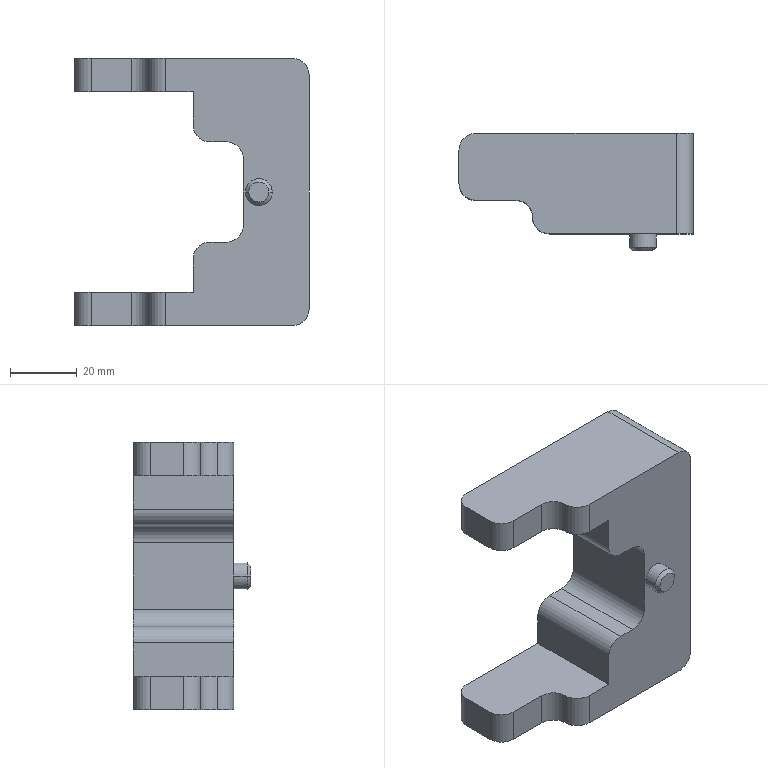Part | NX | features BREP 1 | 1 solid | 36 faces | box 70 x 35 x 80 mm | volume 86102 mm3 | plane 17 | cylinder 16 | cone 3 | commonest cylinder face diameters 10 x14 8 x2
STEP:
#1=CARTESIAN_POINT('',(-8.,0.,30.05));
#2=VERTEX_POINT('',#1);
#3=CARTESIAN_POINT('',(0.3433,0.,30.05));
#4=VERTEX_POINT('',#3);
#5=CARTESIAN_POINT('',(-8.,0.,30.05));
#6=DIRECTION('',(1.,0.,0.));
#7=VECTOR('',#6,1000.);
#8=LINE('',#5,#7);
#9=EDGE_CURVE('',#2,#4,#8,.T.);
#10=ORIENTED_EDGE('',*,*,#9,.T.);
#11=CARTESIAN_POINT('',(0.3433,0.,20.));
#12=VERTEX_POINT('',#11);
#13=CARTESIAN_POINT('',(0.3433,0.,30.05));
#14=DIRECTION('',(0.,0.,-1.));
#15=VECTOR('',#14,1000.);
#16=LINE('',#13,#15);
#17=EDGE_CURVE('',#4,#12,#16,.T.);
#18=ORIENTED_EDGE('',*,*,#17,.T.);
#19=CARTESIAN_POINT('',(5.343,0.,15.));
#20=VERTEX_POINT('',#19);
#21=CARTESIAN_POINT('',(5.343,0.,20.));
#22=DIRECTION('',(0.,-1.,0.));
#23=DIRECTION('',(-1.,0.,0.));
#24=AXIS2_PLACEMENT_3D('',#21,#22,#23);
#25=CIRCLE('',#24,5.);
#26=EDGE_CURVE('',#12,#20,#25,.T.);
#27=ORIENTED_EDGE('',*,*,#26,.T.);
#28=CARTESIAN_POINT('',(10.343,0.,15.));
#29=VERTEX_POINT('',#28);
#30=CARTESIAN_POINT('',(5.343,0.,15.));
#31=DIRECTION('',(1.,0.,0.));
#32=VECTOR('',#31,1000.);
#33=LINE('',#30,#32);
#34=EDGE_CURVE('',#20,#29,#33,.T.);
#35=ORIENTED_EDGE('',*,*,#34,.T.);
#36=CARTESIAN_POINT('',(15.343,0.,10.));
#37=VERTEX_POINT('',#36);
#38=CARTESIAN_POINT('',(10.343,0.,10.));
#39=DIRECTION('',(0.,1.,0.));
#40=DIRECTION('',(0.,0.,1.));
#41=AXIS2_PLACEMENT_3D('',#38,#39,#40);
#42=CIRCLE('',#41,5.);
#43=EDGE_CURVE('',#29,#37,#42,.T.);
#44=ORIENTED_EDGE('',*,*,#43,.T.);
#45=CARTESIAN_POINT('',(15.343,0.,-10.));
#46=VERTEX_POINT('',#45);
#47=CARTESIAN_POINT('',(15.343,0.,10.));
#48=DIRECTION('',(0.,0.,-1.));
#49=VECTOR('',#48,1000.);
#50=LINE('',#47,#49);
#51=EDGE_CURVE('',#37,#46,#50,.T.);
#52=ORIENTED_EDGE('',*,*,#51,.T.);
#53=CARTESIAN_POINT('',(10.343,0.,-15.));
#54=VERTEX_POINT('',#53);
#55=CARTESIAN_POINT('',(10.343,0.,-10.));
#56=DIRECTION('',(0.,1.,0.));
#57=DIRECTION('',(1.,0.,0.));
#58=AXIS2_PLACEMENT_3D('',#55,#56,#57);
#59=CIRCLE('',#58,5.);
#60=EDGE_CURVE('',#46,#54,#59,.T.);
#61=ORIENTED_EDGE('',*,*,#60,.T.);
#62=CARTESIAN_POINT('',(5.343,0.,-15.));
#63=VERTEX_POINT('',#62);
#64=CARTESIAN_POINT('',(10.343,0.,-15.));
#65=DIRECTION('',(-1.,0.,0.));
#66=VECTOR('',#65,1000.);
#67=LINE('',#64,#66);
#68=EDGE_CURVE('',#54,#63,#67,.T.);
#69=ORIENTED_EDGE('',*,*,#68,.T.);
#70=CARTESIAN_POINT('',(0.3433,0.,-20.));
#71=VERTEX_POINT('',#70);
#72=CARTESIAN_POINT('',(5.343,0.,-20.));
#73=DIRECTION('',(0.,-1.,0.));
#74=DIRECTION('',(0.,0.,1.));
#75=AXIS2_PLACEMENT_3D('',#72,#73,#74);
#76=CIRCLE('',#75,5.);
#77=EDGE_CURVE('',#63,#71,#76,.T.);
#78=ORIENTED_EDGE('',*,*,#77,.T.);
#79=CARTESIAN_POINT('',(0.3433,0.,-30.05));
#80=VERTEX_POINT('',#79);
#81=CARTESIAN_POINT('',(0.3433,0.,-20.));
#82=DIRECTION('',(0.,0.,-1.));
#83=VECTOR('',#82,1000.);
#84=LINE('',#81,#83);
#85=EDGE_CURVE('',#71,#80,#84,.T.);
#86=ORIENTED_EDGE('',*,*,#85,.T.);
#87=CARTESIAN_POINT('',(-8.,0.,-30.05));
#88=VERTEX_POINT('',#87);
#89=CARTESIAN_POINT('',(-8.,0.,-30.05));
#90=DIRECTION('',(1.,0.,0.));
#91=VECTOR('',#90,1000.);
#92=LINE('',#89,#91);
#93=EDGE_CURVE('',#88,#80,#92,.T.);
#94=ORIENTED_EDGE('',*,*,#93,.F.);
#95=CARTESIAN_POINT('',(-8.,0.,-40.));
#96=VERTEX_POINT('',#95);
#97=CARTESIAN_POINT('',(-8.,0.,-30.05));
#98=DIRECTION('',(0.,0.,-1.));
#99=VECTOR('',#98,1000.);
#100=LINE('',#97,#99);
#101=EDGE_CURVE('',#88,#96,#100,.T.);
#102=ORIENTED_EDGE('',*,*,#101,.T.);
#103=CARTESIAN_POINT('',(30.,0.,-40.));
#104=VERTEX_POINT('',#103);
#105=CARTESIAN_POINT('',(30.,0.,-40.));
#106=DIRECTION('',(-1.,0.,0.));
#107=VECTOR('',#106,1000.);
#108=LINE('',#105,#107);
#109=EDGE_CURVE('',#104,#96,#108,.T.);
#110=ORIENTED_EDGE('',*,*,#109,.F.);
#111=CARTESIAN_POINT('',(35.,0.,-35.));
#112=VERTEX_POINT('',#111);
#113=CARTESIAN_POINT('',(30.,0.,-35.));
#114=DIRECTION('',(0.,-1.,0.));
#115=DIRECTION('',(0.,0.,-1.));
#116=AXIS2_PLACEMENT_3D('',#113,#114,#115);
#117=CIRCLE('',#116,5.);
#118=EDGE_CURVE('',#104,#112,#117,.T.);
#119=ORIENTED_EDGE('',*,*,#118,.T.);
#120=CARTESIAN_POINT('',(35.,0.,35.));
#121=VERTEX_POINT('',#120);
#122=CARTESIAN_POINT('',(35.,0.,35.));
#123=DIRECTION('',(0.,0.,-1.));
#124=VECTOR('',#123,1000.);
#125=LINE('',#122,#124);
#126=EDGE_CURVE('',#121,#112,#125,.T.);
#127=ORIENTED_EDGE('',*,*,#126,.F.);
#128=CARTESIAN_POINT('',(30.,0.,40.));
#129=VERTEX_POINT('',#128);
#130=CARTESIAN_POINT('',(30.,0.,35.));
#131=DIRECTION('',(0.,-1.,0.));
#132=DIRECTION('',(1.,0.,0.));
#133=AXIS2_PLACEMENT_3D('',#130,#131,#132);
#134=CIRCLE('',#133,5.);
#135=EDGE_CURVE('',#121,#129,#134,.T.);
#136=ORIENTED_EDGE('',*,*,#135,.T.);
#137=CARTESIAN_POINT('',(-8.,0.,40.));
#138=VERTEX_POINT('',#137);
#139=CARTESIAN_POINT('',(-8.,0.,40.));
#140=DIRECTION('',(1.,0.,0.));
#141=VECTOR('',#140,1000.);
#142=LINE('',#139,#141);
#143=EDGE_CURVE('',#138,#129,#142,.T.);
#144=ORIENTED_EDGE('',*,*,#143,.F.);
#145=CARTESIAN_POINT('',(-8.,0.,40.));
#146=DIRECTION('',(0.,0.,-1.));
#147=VECTOR('',#146,1000.);
#148=LINE('',#145,#147);
#149=EDGE_CURVE('',#138,#2,#148,.T.);
#150=ORIENTED_EDGE('',*,*,#149,.T.);
#151=EDGE_LOOP('',(#10,#18,#27,#35,#44,#52,#61,#69,#78,#86,#94,#102,#110,#119,#127,#136,#144,#150));
#152=FACE_BOUND('',#151,.T.);
#153=CARTESIAN_POINT('',(16.,0.,0.));
#154=VERTEX_POINT('',#153);
#155=CARTESIAN_POINT('',(24.,0.,0.));
#156=VERTEX_POINT('',#155);
#157=CARTESIAN_POINT('',(20.,0.,0.));
#158=DIRECTION('',(0.,1.,0.));
#159=DIRECTION('',(-1.,0.,0.));
#160=AXIS2_PLACEMENT_3D('',#157,#158,#159);
#161=CIRCLE('',#160,4.);
#162=EDGE_CURVE('',#154,#156,#161,.T.);
#163=ORIENTED_EDGE('',*,*,#162,.T.);
#164=CARTESIAN_POINT('',(20.,0.,0.));
#165=DIRECTION('',(0.,1.,0.));
#166=DIRECTION('',(1.,0.,0.));
#167=AXIS2_PLACEMENT_3D('',#164,#165,#166);
#168=CIRCLE('',#167,4.);
#169=EDGE_CURVE('',#156,#154,#168,.T.);
#170=ORIENTED_EDGE('',*,*,#169,.T.);
#171=EDGE_LOOP('',(#163,#170));
#172=FACE_BOUND('',#171,.T.);
#173=CARTESIAN_POINT('',(0.,0.,0.));
#174=DIRECTION('',(0.,1.,0.));
#175=DIRECTION('',(1.,0.,0.));
#176=AXIS2_PLACEMENT_3D('',#173,#174,#175);
#177=PLANE('',#176);
#178=ADVANCED_FACE('',(#152,#172),#177,.F.);
#179=CARTESIAN_POINT('',(16.,-4.,0.));
#180=VERTEX_POINT('',#179);
#181=CARTESIAN_POINT('',(16.,0.,0.));
#182=DIRECTION('',(0.000000001,-1.,-0.000000003));
#183=VECTOR('',#182,1000.);
#184=LINE('',#181,#183);
#185=EDGE_CURVE('',#154,#180,#184,.T.);
#186=ORIENTED_EDGE('',*,*,#185,.F.);
#187=ORIENTED_EDGE('',*,*,#169,.F.);
#188=CARTESIAN_POINT('',(24.,-4.,0.));
#189=VERTEX_POINT('',#188);
#190=CARTESIAN_POINT('',(24.,0.,0.));
#191=DIRECTION('',(-0.000000001,-1.,0.000000003));
#192=VECTOR('',#191,1000.);
#193=LINE('',#190,#192);
#194=EDGE_CURVE('',#156,#189,#193,.T.);
#195=ORIENTED_EDGE('',*,*,#194,.T.);
#196=CARTESIAN_POINT('',(20.,-4.,-4.));
#197=VERTEX_POINT('',#196);
#198=CARTESIAN_POINT('',(20.,-4.,0.));
#199=DIRECTION('',(0.,-1.,0.));
#200=DIRECTION('',(-1.,0.,0.));
#201=AXIS2_PLACEMENT_3D('',#198,#199,#200);
#202=CIRCLE('',#201,4.);
#203=EDGE_CURVE('',#197,#189,#202,.T.);
#204=ORIENTED_EDGE('',*,*,#203,.F.);
#205=CARTESIAN_POINT('',(20.,-4.,0.));
#206=DIRECTION('',(0.,-1.,0.));
#207=DIRECTION('',(-1.,0.,0.));
#208=AXIS2_PLACEMENT_3D('',#205,#206,#207);
#209=CIRCLE('',#208,4.);
#210=EDGE_CURVE('',#180,#197,#209,.T.);
#211=ORIENTED_EDGE('',*,*,#210,.F.);
#212=EDGE_LOOP('',(#186,#187,#195,#204,#211));
#213=FACE_BOUND('',#212,.T.);
#214=CARTESIAN_POINT('',(20.,15.,0.));
#215=DIRECTION('',(0.,1.,0.));
#216=DIRECTION('',(1.,0.,0.));
#217=AXIS2_PLACEMENT_3D('',#214,#215,#216);
#218=CYLINDRICAL_SURFACE('',#217,4.);
#219=ADVANCED_FACE('',(#213),#218,.T.);
#220=CARTESIAN_POINT('',(20.,-5.,-3.));
#221=VERTEX_POINT('',#220);
#222=CARTESIAN_POINT('',(20.,-4.5,-3.5));
#223=DIRECTION('',(0.,0.7071,-0.7071));
#224=VECTOR('',#223,1000.);
#225=LINE('',#222,#224);
#226=EDGE_CURVE('',#221,#197,#225,.T.);
#227=ORIENTED_EDGE('',*,*,#226,.F.);
#228=CARTESIAN_POINT('',(17.,-5.,0.));
#229=VERTEX_POINT('',#228);
#230=CARTESIAN_POINT('',(20.,-5.,0.));
#231=DIRECTION('',(0.,-1.,0.));
#232=DIRECTION('',(-1.,0.,0.));
#233=AXIS2_PLACEMENT_3D('',#230,#231,#232);
#234=CIRCLE('',#233,3.);
#235=EDGE_CURVE('',#229,#221,#234,.T.);
#236=ORIENTED_EDGE('',*,*,#235,.F.);
#237=CARTESIAN_POINT('',(17.,-5.,-0.000000013));
#238=DIRECTION('',(-0.7071,0.7071,0.));
#239=VECTOR('',#238,1000.);
#240=LINE('',#237,#239);
#241=EDGE_CURVE('',#229,#180,#240,.T.);
#242=ORIENTED_EDGE('',*,*,#241,.T.);
#243=ORIENTED_EDGE('',*,*,#210,.T.);
#244=EDGE_LOOP('',(#227,#236,#242,#243));
#245=FACE_BOUND('',#244,.T.);
#246=CARTESIAN_POINT('',(20.,-4.5,0.));
#247=DIRECTION('',(0.,1.,0.));
#248=DIRECTION('',(0.,0.,-1.));
#249=AXIS2_PLACEMENT_3D('',#246,#247,#248);
#250=CONICAL_SURFACE('',#249,3.5,0.7854);
#251=ADVANCED_FACE('',(#245),#250,.T.);
#252=ORIENTED_EDGE('',*,*,#235,.T.);
#253=CARTESIAN_POINT('',(23.,-5.,0.));
#254=VERTEX_POINT('',#253);
#255=CARTESIAN_POINT('',(20.,-5.,0.));
#256=DIRECTION('',(0.,-1.,0.));
#257=DIRECTION('',(-1.,0.,0.));
#258=AXIS2_PLACEMENT_3D('',#255,#256,#257);
#259=CIRCLE('',#258,3.);
#260=EDGE_CURVE('',#221,#254,#259,.T.);
#261=ORIENTED_EDGE('',*,*,#260,.T.);
#262=CARTESIAN_POINT('',(20.,-5.,0.));
#263=DIRECTION('',(0.,-1.,0.));
#264=DIRECTION('',(1.,0.,0.));
#265=AXIS2_PLACEMENT_3D('',#262,#263,#264);
#266=CIRCLE('',#265,3.);
#267=EDGE_CURVE('',#254,#229,#266,.T.);
#268=ORIENTED_EDGE('',*,*,#267,.T.);
#269=EDGE_LOOP('',(#252,#261,#268));
#270=FACE_BOUND('',#269,.T.);
#271=CARTESIAN_POINT('',(0.,-5.,0.));
#272=DIRECTION('',(0.,1.,0.));
#273=DIRECTION('',(1.,0.,0.));
#274=AXIS2_PLACEMENT_3D('',#271,#272,#273);
#275=PLANE('',#274);
#276=ADVANCED_FACE('',(#270),#275,.F.);
#277=CARTESIAN_POINT('',(23.,-5.,0.000000013));
#278=DIRECTION('',(0.7071,0.7071,0.));
#279=VECTOR('',#278,1000.);
#280=LINE('',#277,#279);
#281=EDGE_CURVE('',#254,#189,#280,.T.);
#282=ORIENTED_EDGE('',*,*,#281,.T.);
#283=CARTESIAN_POINT('',(20.,-4.,0.));
#284=DIRECTION('',(0.,-1.,0.));
#285=DIRECTION('',(1.,0.,0.));
#286=AXIS2_PLACEMENT_3D('',#283,#284,#285);
#287=CIRCLE('',#286,4.);
#288=EDGE_CURVE('',#189,#180,#287,.T.);
#289=ORIENTED_EDGE('',*,*,#288,.T.);
#290=ORIENTED_EDGE('',*,*,#241,.F.);
#291=ORIENTED_EDGE('',*,*,#267,.F.);
#292=EDGE_LOOP('',(#282,#289,#290,#291));
#293=FACE_BOUND('',#292,.T.);
#294=CARTESIAN_POINT('',(20.,-4.5,0.));
#295=DIRECTION('',(0.,1.,0.));
#296=DIRECTION('',(0.,0.,-1.));
#297=AXIS2_PLACEMENT_3D('',#294,#295,#296);
#298=CONICAL_SURFACE('',#297,3.5,0.7854);
#299=ADVANCED_FACE('',(#293),#298,.T.);
#300=ORIENTED_EDGE('',*,*,#194,.F.);
#301=ORIENTED_EDGE('',*,*,#162,.F.);
#302=ORIENTED_EDGE('',*,*,#185,.T.);
#303=ORIENTED_EDGE('',*,*,#288,.F.);
#304=EDGE_LOOP('',(#300,#301,#302,#303));
#305=FACE_BOUND('',#304,.T.);
#306=CARTESIAN_POINT('',(20.,15.,0.));
#307=DIRECTION('',(0.,1.,0.));
#308=DIRECTION('',(1.,0.,0.));
#309=AXIS2_PLACEMENT_3D('',#306,#307,#308);
#310=CYLINDRICAL_SURFACE('',#309,4.);
#311=ADVANCED_FACE('',(#305),#310,.T.);
#312=ORIENTED_EDGE('',*,*,#149,.F.);
#313=CARTESIAN_POINT('',(-13.,5.,40.));
#314=VERTEX_POINT('',#313);
#315=CARTESIAN_POINT('',(-8.,5.,40.));
#316=DIRECTION('',(0.,0.,1.));
#317=DIRECTION('',(-1.,0.,0.));
#318=AXIS2_PLACEMENT_3D('',#315,#316,#317);
#319=CIRCLE('',#318,5.);
#320=EDGE_CURVE('',#314,#138,#319,.T.);
#321=ORIENTED_EDGE('',*,*,#320,.F.);
#322=CARTESIAN_POINT('',(-13.,5.,30.05));
#323=VERTEX_POINT('',#322);
#324=CARTESIAN_POINT('',(-13.,5.,40.));
#325=DIRECTION('',(0.,0.,-1.));
#326=VECTOR('',#325,1000.);
#327=LINE('',#324,#326);
#328=EDGE_CURVE('',#314,#323,#327,.T.);
#329=ORIENTED_EDGE('',*,*,#328,.T.);
#330=CARTESIAN_POINT('',(-8.,5.,30.05));
#331=DIRECTION('',(0.,0.,-1.));
#332=DIRECTION('',(0.,-1.,0.));
#333=AXIS2_PLACEMENT_3D('',#330,#331,#332);
#334=CIRCLE('',#333,5.);
#335=EDGE_CURVE('',#2,#323,#334,.T.);
#336=ORIENTED_EDGE('',*,*,#335,.F.);
#337=EDGE_LOOP('',(#312,#321,#329,#336));
#338=FACE_BOUND('',#337,.T.);
#339=CARTESIAN_POINT('',(-8.,5.,144.288));
#340=DIRECTION('',(0.,0.,-1.));
#341=DIRECTION('',(0.,-1.,0.));
#342=AXIS2_PLACEMENT_3D('',#339,#340,#341);
#343=CYLINDRICAL_SURFACE('',#342,5.);
#344=ADVANCED_FACE('',(#338),#343,.T.);
#345=CARTESIAN_POINT('',(-18.,10.,30.05));
#346=VERTEX_POINT('',#345);
#347=CARTESIAN_POINT('',(-18.,5.,30.05));
#348=DIRECTION('',(0.,0.,1.));
#349=DIRECTION('',(1.,0.,0.));
#350=AXIS2_PLACEMENT_3D('',#347,#348,#349);
#351=CIRCLE('',#350,5.);
#352=EDGE_CURVE('',#323,#346,#351,.T.);
#353=ORIENTED_EDGE('',*,*,#352,.T.);
#354=CARTESIAN_POINT('',(-30.,10.,30.05));
#355=VERTEX_POINT('',#354);
#356=CARTESIAN_POINT('',(-30.,10.,30.05));
#357=DIRECTION('',(1.,0.,0.));
#358=VECTOR('',#357,1000.);
#359=LINE('',#356,#358);
#360=EDGE_CURVE('',#355,#346,#359,.T.);
#361=ORIENTED_EDGE('',*,*,#360,.F.);
#362=CARTESIAN_POINT('',(-35.,15.,30.05));
#363=VERTEX_POINT('',#362);
#364=CARTESIAN_POINT('',(-30.,15.,30.05));
#365=DIRECTION('',(0.,0.,-1.));
#366=DIRECTION('',(0.,-1.,0.));
#367=AXIS2_PLACEMENT_3D('',#364,#365,#366);
#368=CIRCLE('',#367,5.);
#369=EDGE_CURVE('',#355,#363,#368,.T.);
#370=ORIENTED_EDGE('',*,*,#369,.T.);
#371=CARTESIAN_POINT('',(-35.,25.,30.05));
#372=VERTEX_POINT('',#371);
#373=CARTESIAN_POINT('',(-35.,15.,30.05));
#374=DIRECTION('',(0.,1.,0.));
#375=VECTOR('',#374,1000.);
#376=LINE('',#373,#375);
#377=EDGE_CURVE('',#363,#372,#376,.T.);
#378=ORIENTED_EDGE('',*,*,#377,.T.);
#379=CARTESIAN_POINT('',(-30.,30.,30.05));
#380=VERTEX_POINT('',#379);
#381=CARTESIAN_POINT('',(-30.,25.,30.05));
#382=DIRECTION('',(0.,0.,-1.));
#383=DIRECTION('',(-1.,0.,0.));
#384=AXIS2_PLACEMENT_3D('',#381,#382,#383);
#385=CIRCLE('',#384,5.);
#386=EDGE_CURVE('',#372,#380,#385,.T.);
#387=ORIENTED_EDGE('',*,*,#386,.T.);
#388=CARTESIAN_POINT('',(0.3433,30.,30.05));
#389=VERTEX_POINT('',#388);
#390=CARTESIAN_POINT('',(-30.,30.,30.05));
#391=DIRECTION('',(1.,0.,0.));
#392=VECTOR('',#391,1000.);
#393=LINE('',#390,#392);
#394=EDGE_CURVE('',#380,#389,#393,.T.);
#395=ORIENTED_EDGE('',*,*,#394,.T.);
#396=CARTESIAN_POINT('',(0.3433,30.,30.05));
#397=DIRECTION('',(0.,-1.,0.));
#398=VECTOR('',#397,1000.);
#399=LINE('',#396,#398);
#400=EDGE_CURVE('',#389,#4,#399,.T.);
#401=ORIENTED_EDGE('',*,*,#400,.T.);
#402=ORIENTED_EDGE('',*,*,#9,.F.);
#403=ORIENTED_EDGE('',*,*,#335,.T.);
#404=EDGE_LOOP('',(#353,#361,#370,#378,#387,#395,#401,#402,#403));
#405=FACE_BOUND('',#404,.T.);
#406=CARTESIAN_POINT('',(-35.,30.,30.05));
#407=DIRECTION('',(0.,0.,1.));
#408=DIRECTION('',(1.,0.,0.));
#409=AXIS2_PLACEMENT_3D('',#406,#407,#408);
#410=PLANE('',#409);
#411=ADVANCED_FACE('',(#405),#410,.F.);
#412=CARTESIAN_POINT('',(0.3433,30.,-20.));
#413=VERTEX_POINT('',#412);
#414=CARTESIAN_POINT('',(0.3433,30.,-30.05));
#415=VERTEX_POINT('',#414);
#416=CARTESIAN_POINT('',(0.3433,30.,-20.));
#417=DIRECTION('',(0.,0.,-1.));
#418=VECTOR('',#417,1000.);
#419=LINE('',#416,#418);
#420=EDGE_CURVE('',#413,#415,#419,.T.);
#421=ORIENTED_EDGE('',*,*,#420,.T.);
#422=CARTESIAN_POINT('',(0.3433,30.,-30.05));
#423=DIRECTION('',(0.,-1.,0.));
#424=VECTOR('',#423,1000.);
#425=LINE('',#422,#424);
#426=EDGE_CURVE('',#415,#80,#425,.T.);
#427=ORIENTED_EDGE('',*,*,#426,.T.);
#428=ORIENTED_EDGE('',*,*,#85,.F.);
#429=CARTESIAN_POINT('',(0.3433,0.,-20.));
#430=DIRECTION('',(0.,1.,0.));
#431=VECTOR('',#430,1000.);
#432=LINE('',#429,#431);
#433=EDGE_CURVE('',#71,#413,#432,.T.);
#434=ORIENTED_EDGE('',*,*,#433,.T.);
#435=EDGE_LOOP('',(#421,#427,#428,#434));
#436=FACE_BOUND('',#435,.T.);
#437=CARTESIAN_POINT('',(0.3433,30.,30.05));
#438=DIRECTION('',(1.,0.,0.));
#439=DIRECTION('',(0.,1.,0.));
#440=AXIS2_PLACEMENT_3D('',#437,#438,#439);
#441=PLANE('',#440);
#442=ADVANCED_FACE('',(#436),#441,.F.);
#443=ORIENTED_EDGE('',*,*,#17,.F.);
#444=ORIENTED_EDGE('',*,*,#400,.F.);
#445=CARTESIAN_POINT('',(0.3433,30.,20.));
#446=VERTEX_POINT('',#445);
#447=CARTESIAN_POINT('',(0.3433,30.,30.05));
#448=DIRECTION('',(0.,0.,-1.));
#449=VECTOR('',#448,1000.);
#450=LINE('',#447,#449);
#451=EDGE_CURVE('',#389,#446,#450,.T.);
#452=ORIENTED_EDGE('',*,*,#451,.T.);
#453=CARTESIAN_POINT('',(0.3433,30.,20.));
#454=DIRECTION('',(0.,-1.,0.));
#455=VECTOR('',#454,1000.);
#456=LINE('',#453,#455);
#457=EDGE_CURVE('',#446,#12,#456,.T.);
#458=ORIENTED_EDGE('',*,*,#457,.T.);
#459=EDGE_LOOP('',(#443,#444,#452,#458));
#460=FACE_BOUND('',#459,.T.);
#461=CARTESIAN_POINT('',(0.3433,30.,30.05));
#462=DIRECTION('',(1.,0.,0.));
#463=DIRECTION('',(0.,1.,0.));
#464=AXIS2_PLACEMENT_3D('',#461,#462,#463);
#465=PLANE('',#464);
#466=ADVANCED_FACE('',(#460),#465,.F.);
#467=ORIENTED_EDGE('',*,*,#433,.F.);
#468=ORIENTED_EDGE('',*,*,#77,.F.);
#469=CARTESIAN_POINT('',(5.343,30.,-15.));
#470=VERTEX_POINT('',#469);
#471=CARTESIAN_POINT('',(5.343,0.,-15.));
#472=DIRECTION('',(0.,1.,0.));
#473=VECTOR('',#472,1000.);
#474=LINE('',#471,#473);
#475=EDGE_CURVE('',#63,#470,#474,.T.);
#476=ORIENTED_EDGE('',*,*,#475,.T.);
#477=CARTESIAN_POINT('',(5.343,30.,-20.));
#478=DIRECTION('',(0.,1.,0.));
#479=DIRECTION('',(-1.,0.,0.));
#480=AXIS2_PLACEMENT_3D('',#477,#478,#479);
#481=CIRCLE('',#480,5.);
#482=EDGE_CURVE('',#413,#470,#481,.T.);
#483=ORIENTED_EDGE('',*,*,#482,.F.);
#484=EDGE_LOOP('',(#467,#468,#476,#483));
#485=FACE_BOUND('',#484,.T.);
#486=CARTESIAN_POINT('',(5.343,-50.626,-20.));
#487=DIRECTION('',(0.,1.,0.));
#488=DIRECTION('',(-1.,0.,0.));
#489=AXIS2_PLACEMENT_3D('',#486,#487,#488);
#490=CYLINDRICAL_SURFACE('',#489,5.);
#491=ADVANCED_FACE('',(#485),#490,.T.);
#492=CARTESIAN_POINT('',(-30.,30.,-30.05));
#493=VERTEX_POINT('',#492);
#494=CARTESIAN_POINT('',(-30.,30.,-30.05));
#495=DIRECTION('',(1.,0.,0.));
#496=VECTOR('',#495,1000.);
#497=LINE('',#494,#496);
#498=EDGE_CURVE('',#493,#415,#497,.T.);
#499=ORIENTED_EDGE('',*,*,#498,.T.);
#500=ORIENTED_EDGE('',*,*,#420,.F.);
#501=ORIENTED_EDGE('',*,*,#482,.T.);
#502=CARTESIAN_POINT('',(10.343,30.,-15.));
#503=VERTEX_POINT('',#502);
#504=CARTESIAN_POINT('',(10.343,30.,-15.));
#505=DIRECTION('',(-1.,0.,0.));
#506=VECTOR('',#505,1000.);
#507=LINE('',#504,#506);
#508=EDGE_CURVE('',#503,#470,#507,.T.);
#509=ORIENTED_EDGE('',*,*,#508,.F.);
#510=CARTESIAN_POINT('',(15.343,30.,-10.));
#511=VERTEX_POINT('',#510);
#512=CARTESIAN_POINT('',(10.343,30.,-10.));
#513=DIRECTION('',(0.,-1.,0.));
#514=DIRECTION('',(0.,0.,-1.));
#515=AXIS2_PLACEMENT_3D('',#512,#513,#514);
#516=CIRCLE('',#515,5.);
#517=EDGE_CURVE('',#503,#511,#516,.T.);
#518=ORIENTED_EDGE('',*,*,#517,.T.);
#519=CARTESIAN_POINT('',(15.343,30.,10.));
#520=VERTEX_POINT('',#519);
#521=CARTESIAN_POINT('',(15.343,30.,10.));
#522=DIRECTION('',(0.,0.,-1.));
#523=VECTOR('',#522,1000.);
#524=LINE('',#521,#523);
#525=EDGE_CURVE('',#520,#511,#524,.T.);
#526=ORIENTED_EDGE('',*,*,#525,.F.);
#527=CARTESIAN_POINT('',(10.343,30.,15.));
#528=VERTEX_POINT('',#527);
#529=CARTESIAN_POINT('',(10.343,30.,10.));
#530=DIRECTION('',(0.,-1.,0.));
#531=DIRECTION('',(1.,0.,0.));
#532=AXIS2_PLACEMENT_3D('',#529,#530,#531);
#533=CIRCLE('',#532,5.);
#534=EDGE_CURVE('',#520,#528,#533,.T.);
#535=ORIENTED_EDGE('',*,*,#534,.T.);
#536=CARTESIAN_POINT('',(5.343,30.,15.));
#537=VERTEX_POINT('',#536);
#538=CARTESIAN_POINT('',(5.343,30.,15.));
#539=DIRECTION('',(1.,0.,0.));
#540=VECTOR('',#539,1000.);
#541=LINE('',#538,#540);
#542=EDGE_CURVE('',#537,#528,#541,.T.);
#543=ORIENTED_EDGE('',*,*,#542,.F.);
#544=CARTESIAN_POINT('',(5.343,30.,20.));
#545=DIRECTION('',(0.,1.,0.));
#546=DIRECTION('',(0.,0.,-1.));
#547=AXIS2_PLACEMENT_3D('',#544,#545,#546);
#548=CIRCLE('',#547,5.);
#549=EDGE_CURVE('',#537,#446,#548,.T.);
#550=ORIENTED_EDGE('',*,*,#549,.T.);
#551=ORIENTED_EDGE('',*,*,#451,.F.);
#552=ORIENTED_EDGE('',*,*,#394,.F.);
#553=CARTESIAN_POINT('',(-30.,30.,40.));
#554=VERTEX_POINT('',#553);
#555=CARTESIAN_POINT('',(-30.,30.,30.05));
#556=DIRECTION('',(0.,0.,1.));
#557=VECTOR('',#556,1000.);
#558=LINE('',#555,#557);
#559=EDGE_CURVE('',#380,#554,#558,.T.);
#560=ORIENTED_EDGE('',*,*,#559,.T.);
#561=CARTESIAN_POINT('',(30.,30.,40.));
#562=VERTEX_POINT('',#561);
#563=CARTESIAN_POINT('',(30.,30.,40.));
#564=DIRECTION('',(-1.,0.,0.));
#565=VECTOR('',#564,1000.);
#566=LINE('',#563,#565);
#567=EDGE_CURVE('',#562,#554,#566,.T.);
#568=ORIENTED_EDGE('',*,*,#567,.F.);
#569=CARTESIAN_POINT('',(35.,30.,35.));
#570=VERTEX_POINT('',#569);
#571=CARTESIAN_POINT('',(30.,30.,35.));
#572=DIRECTION('',(0.,1.,0.));
#573=DIRECTION('',(0.,0.,1.));
#574=AXIS2_PLACEMENT_3D('',#571,#572,#573);
#575=CIRCLE('',#574,5.);
#576=EDGE_CURVE('',#562,#570,#575,.T.);
#577=ORIENTED_EDGE('',*,*,#576,.T.);
#578=CARTESIAN_POINT('',(35.,30.,-35.));
#579=VERTEX_POINT('',#578);
#580=CARTESIAN_POINT('',(35.,30.,35.));
#581=DIRECTION('',(0.,0.,-1.));
#582=VECTOR('',#581,1000.);
#583=LINE('',#580,#582);
#584=EDGE_CURVE('',#570,#579,#583,.T.);
#585=ORIENTED_EDGE('',*,*,#584,.T.);
#586=CARTESIAN_POINT('',(30.,30.,-40.));
#587=VERTEX_POINT('',#586);
#588=CARTESIAN_POINT('',(30.,30.,-35.));
#589=DIRECTION('',(0.,1.,0.));
#590=DIRECTION('',(1.,0.,0.));
#591=AXIS2_PLACEMENT_3D('',#588,#589,#590);
#592=CIRCLE('',#591,5.);
#593=EDGE_CURVE('',#579,#587,#592,.T.);
#594=ORIENTED_EDGE('',*,*,#593,.T.);
#595=CARTESIAN_POINT('',(-30.,30.,-40.));
#596=VERTEX_POINT('',#595);
#597=CARTESIAN_POINT('',(-30.,30.,-40.));
#598=DIRECTION('',(1.,0.,0.));
#599=VECTOR('',#598,1000.);
#600=LINE('',#597,#599);
#601=EDGE_CURVE('',#596,#587,#600,.T.);
#602=ORIENTED_EDGE('',*,*,#601,.F.);
#603=CARTESIAN_POINT('',(-30.,30.,-40.));
#604=DIRECTION('',(0.,0.,1.));
#605=VECTOR('',#604,1000.);
#606=LINE('',#603,#605);
#607=EDGE_CURVE('',#596,#493,#606,.T.);
#608=ORIENTED_EDGE('',*,*,#607,.T.);
#609=EDGE_LOOP('',(#499,#500,#501,#509,#518,#526,#535,#543,#550,#551,#552,#560,#568,#577,#585,#594,#602,#608));
#610=FACE_BOUND('',#609,.T.);
#611=CARTESIAN_POINT('',(0.,30.,0.));
#612=DIRECTION('',(0.,1.,0.));
#613=DIRECTION('',(1.,0.,0.));
#614=AXIS2_PLACEMENT_3D('',#611,#612,#613);
#615=PLANE('',#614);
#616=ADVANCED_FACE('',(#610),#615,.T.);
#617=ORIENTED_EDGE('',*,*,#607,.F.);
#618=CARTESIAN_POINT('',(-35.,25.,-40.));
#619=VERTEX_POINT('',#618);
#620=CARTESIAN_POINT('',(-30.,25.,-40.));
#621=DIRECTION('',(0.,0.,-1.));
#622=DIRECTION('',(-1.,0.,0.));
#623=AXIS2_PLACEMENT_3D('',#620,#621,#622);
#624=CIRCLE('',#623,5.);
#625=EDGE_CURVE('',#619,#596,#624,.T.);
#626=ORIENTED_EDGE('',*,*,#625,.F.);
#627=CARTESIAN_POINT('',(-35.,25.,-30.05));
#628=VERTEX_POINT('',#627);
#629=CARTESIAN_POINT('',(-35.,25.,-40.));
#630=DIRECTION('',(0.,0.,1.));
#631=VECTOR('',#630,1000.);
#632=LINE('',#629,#631);
#633=EDGE_CURVE('',#619,#628,#632,.T.);
#634=ORIENTED_EDGE('',*,*,#633,.T.);
#635=CARTESIAN_POINT('',(-30.,25.,-30.05));
#636=DIRECTION('',(0.,0.,1.));
#637=DIRECTION('',(0.,1.,0.));
#638=AXIS2_PLACEMENT_3D('',#635,#636,#637);
#639=CIRCLE('',#638,5.);
#640=EDGE_CURVE('',#493,#628,#639,.T.);
#641=ORIENTED_EDGE('',*,*,#640,.F.);
#642=EDGE_LOOP('',(#617,#626,#634,#641));
#643=FACE_BOUND('',#642,.T.);
#644=CARTESIAN_POINT('',(-30.,25.,-144.288));
#645=DIRECTION('',(0.,0.,1.));
#646=DIRECTION('',(0.,1.,0.));
#647=AXIS2_PLACEMENT_3D('',#644,#645,#646);
#648=CYLINDRICAL_SURFACE('',#647,5.);
#649=ADVANCED_FACE('',(#643),#648,.T.);
#650=ORIENTED_EDGE('',*,*,#93,.T.);
#651=ORIENTED_EDGE('',*,*,#426,.F.);
#652=ORIENTED_EDGE('',*,*,#498,.F.);
#653=ORIENTED_EDGE('',*,*,#640,.T.);
#654=CARTESIAN_POINT('',(-35.,15.,-30.05));
#655=VERTEX_POINT('',#654);
#656=CARTESIAN_POINT('',(-35.,15.,-30.05));
#657=DIRECTION('',(0.,1.,0.));
#658=VECTOR('',#657,1000.);
#659=LINE('',#656,#658);
#660=EDGE_CURVE('',#655,#628,#659,.T.);
#661=ORIENTED_EDGE('',*,*,#660,.F.);
#662=CARTESIAN_POINT('',(-30.,10.,-30.05));
#663=VERTEX_POINT('',#662);
#664=CARTESIAN_POINT('',(-30.,15.,-30.05));
#665=DIRECTION('',(0.,0.,1.));
#666=DIRECTION('',(-1.,0.,0.));
#667=AXIS2_PLACEMENT_3D('',#664,#665,#666);
#668=CIRCLE('',#667,5.);
#669=EDGE_CURVE('',#655,#663,#668,.T.);
#670=ORIENTED_EDGE('',*,*,#669,.T.);
#671=CARTESIAN_POINT('',(-18.,10.,-30.05));
#672=VERTEX_POINT('',#671);
#673=CARTESIAN_POINT('',(-30.,10.,-30.05));
#674=DIRECTION('',(1.,0.,0.));
#675=VECTOR('',#674,1000.);
#676=LINE('',#673,#675);
#677=EDGE_CURVE('',#663,#672,#676,.T.);
#678=ORIENTED_EDGE('',*,*,#677,.T.);
#679=CARTESIAN_POINT('',(-13.,5.,-30.05));
#680=VERTEX_POINT('',#679);
#681=CARTESIAN_POINT('',(-18.,5.,-30.05));
#682=DIRECTION('',(0.,0.,-1.));
#683=DIRECTION('',(0.,1.,0.));
#684=AXIS2_PLACEMENT_3D('',#681,#682,#683);
#685=CIRCLE('',#684,5.);
#686=EDGE_CURVE('',#672,#680,#685,.T.);
#687=ORIENTED_EDGE('',*,*,#686,.T.);
#688=CARTESIAN_POINT('',(-8.,5.,-30.05));
#689=DIRECTION('',(0.,0.,1.));
#690=DIRECTION('',(-1.,0.,0.));
#691=AXIS2_PLACEMENT_3D('',#688,#689,#690);
#692=CIRCLE('',#691,5.);
#693=EDGE_CURVE('',#680,#88,#692,.T.);
#694=ORIENTED_EDGE('',*,*,#693,.T.);
#695=EDGE_LOOP('',(#650,#651,#652,#653,#661,#670,#678,#687,#694));
#696=FACE_BOUND('',#695,.T.);
#697=CARTESIAN_POINT('',(0.3433,30.,-30.05));
#698=DIRECTION('',(0.,0.,-1.));
#699=DIRECTION('',(0.,-1.,0.));
#700=AXIS2_PLACEMENT_3D('',#697,#698,#699);
#701=PLANE('',#700);
#702=ADVANCED_FACE('',(#696),#701,.F.);
#703=ORIENTED_EDGE('',*,*,#101,.F.);
#704=ORIENTED_EDGE('',*,*,#693,.F.);
#705=CARTESIAN_POINT('',(-13.,5.,-40.));
#706=VERTEX_POINT('',#705);
#707=CARTESIAN_POINT('',(-13.,5.,-30.05));
#708=DIRECTION('',(0.,0.,-1.));
#709=VECTOR('',#708,1000.);
#710=LINE('',#707,#709);
#711=EDGE_CURVE('',#680,#706,#710,.T.);
#712=ORIENTED_EDGE('',*,*,#711,.T.);
#713=CARTESIAN_POINT('',(-8.,5.,-40.));
#714=DIRECTION('',(0.,0.,-1.));
#715=DIRECTION('',(0.,-1.,0.));
#716=AXIS2_PLACEMENT_3D('',#713,#714,#715);
#717=CIRCLE('',#716,5.);
#718=EDGE_CURVE('',#96,#706,#717,.T.);
#719=ORIENTED_EDGE('',*,*,#718,.F.);
#720=EDGE_LOOP('',(#703,#704,#712,#719));
#721=FACE_BOUND('',#720,.T.);
#722=CARTESIAN_POINT('',(-8.,5.,144.288));
#723=DIRECTION('',(0.,0.,-1.));
#724=DIRECTION('',(0.,-1.,0.));
#725=AXIS2_PLACEMENT_3D('',#722,#723,#724);
#726=CYLINDRICAL_SURFACE('',#725,5.);
#727=ADVANCED_FACE('',(#721),#726,.T.);
#728=CARTESIAN_POINT('',(-18.,10.,-40.));
#729=VERTEX_POINT('',#728);
#730=CARTESIAN_POINT('',(-18.,5.,-40.));
#731=DIRECTION('',(0.,0.,1.));
#732=DIRECTION('',(1.,0.,0.));
#733=AXIS2_PLACEMENT_3D('',#730,#731,#732);
#734=CIRCLE('',#733,5.);
#735=EDGE_CURVE('',#706,#729,#734,.T.);
#736=ORIENTED_EDGE('',*,*,#735,.T.);
#737=CARTESIAN_POINT('',(-30.,10.,-40.));
#738=VERTEX_POINT('',#737);
#739=CARTESIAN_POINT('',(-30.,10.,-40.));
#740=DIRECTION('',(1.,0.,0.));
#741=VECTOR('',#740,1000.);
#742=LINE('',#739,#741);
#743=EDGE_CURVE('',#738,#729,#742,.T.);
#744=ORIENTED_EDGE('',*,*,#743,.F.);
#745=CARTESIAN_POINT('',(-35.,15.,-40.));
#746=VERTEX_POINT('',#745);
#747=CARTESIAN_POINT('',(-30.,15.,-40.));
#748=DIRECTION('',(0.,0.,-1.));
#749=DIRECTION('',(0.,-1.,0.));
#750=AXIS2_PLACEMENT_3D('',#747,#748,#749);
#751=CIRCLE('',#750,5.);
#752=EDGE_CURVE('',#738,#746,#751,.T.);
#753=ORIENTED_EDGE('',*,*,#752,.T.);
#754=CARTESIAN_POINT('',(-35.,15.,-40.));
#755=DIRECTION('',(0.,1.,0.));
#756=VECTOR('',#755,1000.);
#757=LINE('',#754,#756);
#758=EDGE_CURVE('',#746,#619,#757,.T.);
#759=ORIENTED_EDGE('',*,*,#758,.T.);
#760=ORIENTED_EDGE('',*,*,#625,.T.);
#761=ORIENTED_EDGE('',*,*,#601,.T.);
#762=CARTESIAN_POINT('',(30.,30.,-40.));
#763=DIRECTION('',(0.,-1.,0.));
#764=VECTOR('',#763,1000.);
#765=LINE('',#762,#764);
#766=EDGE_CURVE('',#587,#104,#765,.T.);
#767=ORIENTED_EDGE('',*,*,#766,.T.);
#768=ORIENTED_EDGE('',*,*,#109,.T.);
#769=ORIENTED_EDGE('',*,*,#718,.T.);
#770=EDGE_LOOP('',(#736,#744,#753,#759,#760,#761,#767,#768,#769));
#771=FACE_BOUND('',#770,.T.);
#772=CARTESIAN_POINT('',(35.,0.,-40.));
#773=DIRECTION('',(0.,0.,-1.));
#774=DIRECTION('',(0.,-1.,0.));
#775=AXIS2_PLACEMENT_3D('',#772,#773,#774);
#776=PLANE('',#775);
#777=ADVANCED_FACE('',(#771),#776,.T.);
#778=ORIENTED_EDGE('',*,*,#766,.F.);
#779=ORIENTED_EDGE('',*,*,#593,.F.);
#780=CARTESIAN_POINT('',(35.,30.,-35.));
#781=DIRECTION('',(0.,-1.,0.));
#782=VECTOR('',#781,1000.);
#783=LINE('',#780,#782);
#784=EDGE_CURVE('',#579,#112,#783,.T.);
#785=ORIENTED_EDGE('',*,*,#784,.T.);
#786=ORIENTED_EDGE('',*,*,#118,.F.);
#787=EDGE_LOOP('',(#778,#779,#785,#786));
#788=FACE_BOUND('',#787,.T.);
#789=CARTESIAN_POINT('',(30.,75.626,-35.));
#790=DIRECTION('',(0.,-1.,0.));
#791=DIRECTION('',(0.,0.,-1.));
#792=AXIS2_PLACEMENT_3D('',#789,#790,#791);
#793=CYLINDRICAL_SURFACE('',#792,5.);
#794=ADVANCED_FACE('',(#788),#793,.T.);
#795=ORIENTED_EDGE('',*,*,#584,.F.);
#796=CARTESIAN_POINT('',(35.,30.,35.));
#797=DIRECTION('',(0.,-1.,0.));
#798=VECTOR('',#797,1000.);
#799=LINE('',#796,#798);
#800=EDGE_CURVE('',#570,#121,#799,.T.);
#801=ORIENTED_EDGE('',*,*,#800,.T.);
#802=ORIENTED_EDGE('',*,*,#126,.T.);
#803=ORIENTED_EDGE('',*,*,#784,.F.);
#804=EDGE_LOOP('',(#795,#801,#802,#803));
#805=FACE_BOUND('',#804,.T.);
#806=CARTESIAN_POINT('',(35.,0.,40.));
#807=DIRECTION('',(1.,0.,0.));
#808=DIRECTION('',(0.,1.,0.));
#809=AXIS2_PLACEMENT_3D('',#806,#807,#808);
#810=PLANE('',#809);
#811=ADVANCED_FACE('',(#805),#810,.T.);
#812=ORIENTED_EDGE('',*,*,#800,.F.);
#813=ORIENTED_EDGE('',*,*,#576,.F.);
#814=CARTESIAN_POINT('',(30.,30.,40.));
#815=DIRECTION('',(0.,-1.,0.));
#816=VECTOR('',#815,1000.);
#817=LINE('',#814,#816);
#818=EDGE_CURVE('',#562,#129,#817,.T.);
#819=ORIENTED_EDGE('',*,*,#818,.T.);
#820=ORIENTED_EDGE('',*,*,#135,.F.);
#821=EDGE_LOOP('',(#812,#813,#819,#820));
#822=FACE_BOUND('',#821,.T.);
#823=CARTESIAN_POINT('',(30.,75.626,35.));
#824=DIRECTION('',(0.,-1.,0.));
#825=DIRECTION('',(1.,0.,0.));
#826=AXIS2_PLACEMENT_3D('',#823,#824,#825);
#827=CYLINDRICAL_SURFACE('',#826,5.);
#828=ADVANCED_FACE('',(#822),#827,.T.);
#829=ORIENTED_EDGE('',*,*,#143,.T.);
#830=ORIENTED_EDGE('',*,*,#818,.F.);
#831=ORIENTED_EDGE('',*,*,#567,.T.);
#832=CARTESIAN_POINT('',(-35.,25.,40.));
#833=VERTEX_POINT('',#832);
#834=CARTESIAN_POINT('',(-30.,25.,40.));
#835=DIRECTION('',(0.,0.,1.));
#836=DIRECTION('',(0.,1.,0.));
#837=AXIS2_PLACEMENT_3D('',#834,#835,#836);
#838=CIRCLE('',#837,5.);
#839=EDGE_CURVE('',#554,#833,#838,.T.);
#840=ORIENTED_EDGE('',*,*,#839,.T.);
#841=CARTESIAN_POINT('',(-35.,15.,40.));
#842=VERTEX_POINT('',#841);
#843=CARTESIAN_POINT('',(-35.,15.,40.));
#844=DIRECTION('',(0.,1.,0.));
#845=VECTOR('',#844,1000.);
#846=LINE('',#843,#845);
#847=EDGE_CURVE('',#842,#833,#846,.T.);
#848=ORIENTED_EDGE('',*,*,#847,.F.);
#849=CARTESIAN_POINT('',(-30.,10.,40.));
#850=VERTEX_POINT('',#849);
#851=CARTESIAN_POINT('',(-30.,15.,40.));
#852=DIRECTION('',(0.,0.,1.));
#853=DIRECTION('',(-1.,0.,0.));
#854=AXIS2_PLACEMENT_3D('',#851,#852,#853);
#855=CIRCLE('',#854,5.);
#856=EDGE_CURVE('',#842,#850,#855,.T.);
#857=ORIENTED_EDGE('',*,*,#856,.T.);
#858=CARTESIAN_POINT('',(-18.,10.,40.));
#859=VERTEX_POINT('',#858);
#860=CARTESIAN_POINT('',(-30.,10.,40.));
#861=DIRECTION('',(1.,0.,0.));
#862=VECTOR('',#861,1000.);
#863=LINE('',#860,#862);
#864=EDGE_CURVE('',#850,#859,#863,.T.);
#865=ORIENTED_EDGE('',*,*,#864,.T.);
#866=CARTESIAN_POINT('',(-18.,5.,40.));
#867=DIRECTION('',(0.,0.,-1.));
#868=DIRECTION('',(0.,1.,0.));
#869=AXIS2_PLACEMENT_3D('',#866,#867,#868);
#870=CIRCLE('',#869,5.);
#871=EDGE_CURVE('',#859,#314,#870,.T.);
#872=ORIENTED_EDGE('',*,*,#871,.T.);
#873=ORIENTED_EDGE('',*,*,#320,.T.);
#874=EDGE_LOOP('',(#829,#830,#831,#840,#848,#857,#865,#872,#873));
#875=FACE_BOUND('',#874,.T.);
#876=CARTESIAN_POINT('',(-35.,0.,40.));
#877=DIRECTION('',(0.,0.,1.));
#878=DIRECTION('',(1.,0.,0.));
#879=AXIS2_PLACEMENT_3D('',#876,#877,#878);
#880=PLANE('',#879);
#881=ADVANCED_FACE('',(#875),#880,.T.);
#882=ORIENTED_EDGE('',*,*,#871,.F.);
#883=CARTESIAN_POINT('',(-18.,10.,40.));
#884=DIRECTION('',(0.,0.,-1.));
#885=VECTOR('',#884,1000.);
#886=LINE('',#883,#885);
#887=EDGE_CURVE('',#859,#346,#886,.T.);
#888=ORIENTED_EDGE('',*,*,#887,.T.);
#889=ORIENTED_EDGE('',*,*,#352,.F.);
#890=ORIENTED_EDGE('',*,*,#328,.F.);
#891=EDGE_LOOP('',(#882,#888,#889,#890));
#892=FACE_BOUND('',#891,.T.);
#893=CARTESIAN_POINT('',(-18.,5.,144.288));
#894=DIRECTION('',(0.,0.,-1.));
#895=DIRECTION('',(0.,1.,0.));
#896=AXIS2_PLACEMENT_3D('',#893,#894,#895);
#897=CYLINDRICAL_SURFACE('',#896,5.);
#898=ADVANCED_FACE('',(#892),#897,.F.);
#899=ORIENTED_EDGE('',*,*,#743,.T.);
#900=CARTESIAN_POINT('',(-18.,10.,-30.05));
#901=DIRECTION('',(0.,0.,-1.));
#902=VECTOR('',#901,1000.);
#903=LINE('',#900,#902);
#904=EDGE_CURVE('',#672,#729,#903,.T.);
#905=ORIENTED_EDGE('',*,*,#904,.F.);
#906=ORIENTED_EDGE('',*,*,#677,.F.);
#907=CARTESIAN_POINT('',(-30.,10.,-40.));
#908=DIRECTION('',(0.,0.,1.));
#909=VECTOR('',#908,1000.);
#910=LINE('',#907,#909);
#911=EDGE_CURVE('',#738,#663,#910,.T.);
#912=ORIENTED_EDGE('',*,*,#911,.F.);
#913=EDGE_LOOP('',(#899,#905,#906,#912));
#914=FACE_BOUND('',#913,.T.);
#915=CARTESIAN_POINT('',(-13.,10.,40.));
#916=DIRECTION('',(0.,1.,0.));
#917=DIRECTION('',(1.,0.,0.));
#918=AXIS2_PLACEMENT_3D('',#915,#916,#917);
#919=PLANE('',#918);
#920=ADVANCED_FACE('',(#914),#919,.F.);
#921=ORIENTED_EDGE('',*,*,#360,.T.);
#922=ORIENTED_EDGE('',*,*,#887,.F.);
#923=ORIENTED_EDGE('',*,*,#864,.F.);
#924=CARTESIAN_POINT('',(-30.,10.,30.05));
#925=DIRECTION('',(0.,0.,1.));
#926=VECTOR('',#925,1000.);
#927=LINE('',#924,#926);
#928=EDGE_CURVE('',#355,#850,#927,.T.);
#929=ORIENTED_EDGE('',*,*,#928,.F.);
#930=EDGE_LOOP('',(#921,#922,#923,#929));
#931=FACE_BOUND('',#930,.T.);
#932=CARTESIAN_POINT('',(-13.,10.,40.));
#933=DIRECTION('',(0.,1.,0.));
#934=DIRECTION('',(1.,0.,0.));
#935=AXIS2_PLACEMENT_3D('',#932,#933,#934);
#936=PLANE('',#935);
#937=ADVANCED_FACE('',(#931),#936,.F.);
#938=CARTESIAN_POINT('',(-35.,15.,-40.));
#939=DIRECTION('',(0.,0.,1.));
#940=VECTOR('',#939,1000.);
#941=LINE('',#938,#940);
#942=EDGE_CURVE('',#746,#655,#941,.T.);
#943=ORIENTED_EDGE('',*,*,#942,.F.);
#944=ORIENTED_EDGE('',*,*,#752,.F.);
#945=ORIENTED_EDGE('',*,*,#911,.T.);
#946=ORIENTED_EDGE('',*,*,#669,.F.);
#947=EDGE_LOOP('',(#943,#944,#945,#946));
#948=FACE_BOUND('',#947,.T.);
#949=CARTESIAN_POINT('',(-30.,15.,-144.288));
#950=DIRECTION('',(0.,0.,1.));
#951=DIRECTION('',(-1.,0.,0.));
#952=AXIS2_PLACEMENT_3D('',#949,#950,#951);
#953=CYLINDRICAL_SURFACE('',#952,5.);
#954=ADVANCED_FACE('',(#948),#953,.T.);
#955=ORIENTED_EDGE('',*,*,#660,.T.);
#956=ORIENTED_EDGE('',*,*,#633,.F.);
#957=ORIENTED_EDGE('',*,*,#758,.F.);
#958=ORIENTED_EDGE('',*,*,#942,.T.);
#959=EDGE_LOOP('',(#955,#956,#957,#958));
#960=FACE_BOUND('',#959,.T.);
#961=CARTESIAN_POINT('',(-35.,0.,-40.));
#962=DIRECTION('',(-1.,0.,0.));
#963=DIRECTION('',(0.,0.,1.));
#964=AXIS2_PLACEMENT_3D('',#961,#962,#963);
#965=PLANE('',#964);
#966=ADVANCED_FACE('',(#960),#965,.T.);
#967=ORIENTED_EDGE('',*,*,#847,.T.);
#968=CARTESIAN_POINT('',(-35.,25.,30.05));
#969=DIRECTION('',(0.,0.,1.));
#970=VECTOR('',#969,1000.);
#971=LINE('',#968,#970);
#972=EDGE_CURVE('',#372,#833,#971,.T.);
#973=ORIENTED_EDGE('',*,*,#972,.F.);
#974=ORIENTED_EDGE('',*,*,#377,.F.);
#975=CARTESIAN_POINT('',(-35.,15.,30.05));
#976=DIRECTION('',(0.,0.,1.));
#977=VECTOR('',#976,1000.);
#978=LINE('',#975,#977);
#979=EDGE_CURVE('',#363,#842,#978,.T.);
#980=ORIENTED_EDGE('',*,*,#979,.T.);
#981=EDGE_LOOP('',(#967,#973,#974,#980));
#982=FACE_BOUND('',#981,.T.);
#983=CARTESIAN_POINT('',(-35.,0.,-40.));
#984=DIRECTION('',(-1.,0.,0.));
#985=DIRECTION('',(0.,0.,1.));
#986=AXIS2_PLACEMENT_3D('',#983,#984,#985);
#987=PLANE('',#986);
#988=ADVANCED_FACE('',(#982),#987,.T.);
#989=ORIENTED_EDGE('',*,*,#979,.F.);
#990=ORIENTED_EDGE('',*,*,#369,.F.);
#991=ORIENTED_EDGE('',*,*,#928,.T.);
#992=ORIENTED_EDGE('',*,*,#856,.F.);
#993=EDGE_LOOP('',(#989,#990,#991,#992));
#994=FACE_BOUND('',#993,.T.);
#995=CARTESIAN_POINT('',(-30.,15.,-144.288));
#996=DIRECTION('',(0.,0.,1.));
#997=DIRECTION('',(-1.,0.,0.));
#998=AXIS2_PLACEMENT_3D('',#995,#996,#997);
#999=CYLINDRICAL_SURFACE('',#998,5.);
#1000=ADVANCED_FACE('',(#994),#999,.T.);
#1001=ORIENTED_EDGE('',*,*,#559,.F.);
#1002=ORIENTED_EDGE('',*,*,#386,.F.);
#1003=ORIENTED_EDGE('',*,*,#972,.T.);
#1004=ORIENTED_EDGE('',*,*,#839,.F.);
#1005=EDGE_LOOP('',(#1001,#1002,#1003,#1004));
#1006=FACE_BOUND('',#1005,.T.);
#1007=CARTESIAN_POINT('',(-30.,25.,-144.288));
#1008=DIRECTION('',(0.,0.,1.));
#1009=DIRECTION('',(0.,1.,0.));
#1010=AXIS2_PLACEMENT_3D('',#1007,#1008,#1009);
#1011=CYLINDRICAL_SURFACE('',#1010,5.);
#1012=ADVANCED_FACE('',(#1006),#1011,.T.);
#1013=ORIENTED_EDGE('',*,*,#686,.F.);
#1014=ORIENTED_EDGE('',*,*,#904,.T.);
#1015=ORIENTED_EDGE('',*,*,#735,.F.);
#1016=ORIENTED_EDGE('',*,*,#711,.F.);
#1017=EDGE_LOOP('',(#1013,#1014,#1015,#1016));
#1018=FACE_BOUND('',#1017,.T.);
#1019=CARTESIAN_POINT('',(-18.,5.,144.288));
#1020=DIRECTION('',(0.,0.,-1.));
#1021=DIRECTION('',(0.,1.,0.));
#1022=AXIS2_PLACEMENT_3D('',#1019,#1020,#1021);
#1023=CYLINDRICAL_SURFACE('',#1022,5.);
#1024=ADVANCED_FACE('',(#1018),#1023,.F.);
#1025=ORIENTED_EDGE('',*,*,#457,.F.);
#1026=ORIENTED_EDGE('',*,*,#549,.F.);
#1027=CARTESIAN_POINT('',(5.343,30.,15.));
#1028=DIRECTION('',(0.,-1.,0.));
#1029=VECTOR('',#1028,1000.);
#1030=LINE('',#1027,#1029);
#1031=EDGE_CURVE('',#537,#20,#1030,.T.);
#1032=ORIENTED_EDGE('',*,*,#1031,.T.);
#1033=ORIENTED_EDGE('',*,*,#26,.F.);
#1034=EDGE_LOOP('',(#1025,#1026,#1032,#1033));
#1035=FACE_BOUND('',#1034,.T.);
#1036=CARTESIAN_POINT('',(5.343,75.626,20.));
#1037=DIRECTION('',(0.,-1.,0.));
#1038=DIRECTION('',(-1.,0.,0.));
#1039=AXIS2_PLACEMENT_3D('',#1036,#1037,#1038);
#1040=CYLINDRICAL_SURFACE('',#1039,5.);
#1041=ADVANCED_FACE('',(#1035),#1040,.T.);
#1042=ORIENTED_EDGE('',*,*,#542,.T.);
#1043=CARTESIAN_POINT('',(10.343,30.,15.));
#1044=DIRECTION('',(0.,-1.,0.));
#1045=VECTOR('',#1044,1000.);
#1046=LINE('',#1043,#1045);
#1047=EDGE_CURVE('',#528,#29,#1046,.T.);
#1048=ORIENTED_EDGE('',*,*,#1047,.T.);
#1049=ORIENTED_EDGE('',*,*,#34,.F.);
#1050=ORIENTED_EDGE('',*,*,#1031,.F.);
#1051=EDGE_LOOP('',(#1042,#1048,#1049,#1050));
#1052=FACE_BOUND('',#1051,.T.);
#1053=CARTESIAN_POINT('',(0.3433,30.,15.));
#1054=DIRECTION('',(0.,0.,1.));
#1055=DIRECTION('',(1.,0.,0.));
#1056=AXIS2_PLACEMENT_3D('',#1053,#1054,#1055);
#1057=PLANE('',#1056);
#1058=ADVANCED_FACE('',(#1052),#1057,.F.);
#1059=ORIENTED_EDGE('',*,*,#43,.F.);
#1060=ORIENTED_EDGE('',*,*,#1047,.F.);
#1061=ORIENTED_EDGE('',*,*,#534,.F.);
#1062=CARTESIAN_POINT('',(15.343,30.,10.));
#1063=DIRECTION('',(0.,-1.,0.));
#1064=VECTOR('',#1063,1000.);
#1065=LINE('',#1062,#1064);
#1066=EDGE_CURVE('',#520,#37,#1065,.T.);
#1067=ORIENTED_EDGE('',*,*,#1066,.T.);
#1068=EDGE_LOOP('',(#1059,#1060,#1061,#1067));
#1069=FACE_BOUND('',#1068,.T.);
#1070=CARTESIAN_POINT('',(10.343,75.626,10.));
#1071=DIRECTION('',(0.,-1.,0.));
#1072=DIRECTION('',(1.,0.,0.));
#1073=AXIS2_PLACEMENT_3D('',#1070,#1071,#1072);
#1074=CYLINDRICAL_SURFACE('',#1073,5.);
#1075=ADVANCED_FACE('',(#1069),#1074,.F.);
#1076=ORIENTED_EDGE('',*,*,#51,.F.);
#1077=ORIENTED_EDGE('',*,*,#1066,.F.);
#1078=ORIENTED_EDGE('',*,*,#525,.T.);
#1079=CARTESIAN_POINT('',(15.343,30.,-10.));
#1080=DIRECTION('',(0.,-1.,0.));
#1081=VECTOR('',#1080,1000.);
#1082=LINE('',#1079,#1081);
#1083=EDGE_CURVE('',#511,#46,#1082,.T.);
#1084=ORIENTED_EDGE('',*,*,#1083,.T.);
#1085=EDGE_LOOP('',(#1076,#1077,#1078,#1084));
#1086=FACE_BOUND('',#1085,.T.);
#1087=CARTESIAN_POINT('',(15.343,30.,15.));
#1088=DIRECTION('',(1.,0.,0.));
#1089=DIRECTION('',(0.,1.,0.));
#1090=AXIS2_PLACEMENT_3D('',#1087,#1088,#1089);
#1091=PLANE('',#1090);
#1092=ADVANCED_FACE('',(#1086),#1091,.F.);
#1093=ORIENTED_EDGE('',*,*,#60,.F.);
#1094=ORIENTED_EDGE('',*,*,#1083,.F.);
#1095=ORIENTED_EDGE('',*,*,#517,.F.);
#1096=CARTESIAN_POINT('',(10.343,30.,-15.));
#1097=DIRECTION('',(0.,-1.,0.));
#1098=VECTOR('',#1097,1000.);
#1099=LINE('',#1096,#1098);
#1100=EDGE_CURVE('',#503,#54,#1099,.T.);
#1101=ORIENTED_EDGE('',*,*,#1100,.T.);
#1102=EDGE_LOOP('',(#1093,#1094,#1095,#1101));
#1103=FACE_BOUND('',#1102,.T.);
#1104=CARTESIAN_POINT('',(10.343,75.626,-10.));
#1105=DIRECTION('',(0.,-1.,0.));
#1106=DIRECTION('',(0.,0.,-1.));
#1107=AXIS2_PLACEMENT_3D('',#1104,#1105,#1106);
#1108=CYLINDRICAL_SURFACE('',#1107,5.);
#1109=ADVANCED_FACE('',(#1103),#1108,.F.);
#1110=ORIENTED_EDGE('',*,*,#68,.F.);
#1111=ORIENTED_EDGE('',*,*,#1100,.F.);
#1112=ORIENTED_EDGE('',*,*,#508,.T.);
#1113=ORIENTED_EDGE('',*,*,#475,.F.);
#1114=EDGE_LOOP('',(#1110,#1111,#1112,#1113));
#1115=FACE_BOUND('',#1114,.T.);
#1116=CARTESIAN_POINT('',(15.343,30.,-15.));
#1117=DIRECTION('',(0.,0.,-1.));
#1118=DIRECTION('',(0.,-1.,0.));
#1119=AXIS2_PLACEMENT_3D('',#1116,#1117,#1118);
#1120=PLANE('',#1119);
#1121=ADVANCED_FACE('',(#1115),#1120,.F.);
#1122=ORIENTED_EDGE('',*,*,#260,.F.);
#1123=ORIENTED_EDGE('',*,*,#226,.T.);
#1124=ORIENTED_EDGE('',*,*,#203,.T.);
#1125=ORIENTED_EDGE('',*,*,#281,.F.);
#1126=EDGE_LOOP('',(#1122,#1123,#1124,#1125));
#1127=FACE_BOUND('',#1126,.T.);
#1128=CARTESIAN_POINT('',(20.,-4.5,0.));
#1129=DIRECTION('',(0.,1.,0.));
#1130=DIRECTION('',(0.,0.,-1.));
#1131=AXIS2_PLACEMENT_3D('',#1128,#1129,#1130);
#1132=CONICAL_SURFACE('',#1131,3.5,0.7854);
#1133=ADVANCED_FACE('',(#1127),#1132,.T.);
#1134=CLOSED_SHELL('',(#178,#219,#251,#276,#299,#311,#344,#411,#442,#466,#491,#616,#649,#702,#727,#777,#794,#811,#828,#881,#898,#920,#937,#954,#966,#988,#1000,#1012,#1024,#1041,#1058,#1075,#1092,#1109,#1121,#1133));
#1135=MANIFOLD_SOLID_BREP('',#1134);
#1136=(LENGTH_UNIT()NAMED_UNIT(*)SI_UNIT(.MILLI.,.METRE.));
#1137=UNCERTAINTY_MEASURE_WITH_UNIT(LENGTH_MEASURE(0.00001),#1136,'','');
#1138=(NAMED_UNIT(*)PLANE_ANGLE_UNIT()SI_UNIT($,.RADIAN.));
#1139=(NAMED_UNIT(*)SI_UNIT($,.STERADIAN.)SOLID_ANGLE_UNIT());
#1140=(GEOMETRIC_REPRESENTATION_CONTEXT(3)GLOBAL_UNCERTAINTY_ASSIGNED_CONTEXT((#1137))GLOBAL_UNIT_ASSIGNED_CONTEXT((#1136,#1138,#1139))REPRESENTATION_CONTEXT('',''));
#1141=ADVANCED_BREP_SHAPE_REPRESENTATION('',(#1135),#1140);